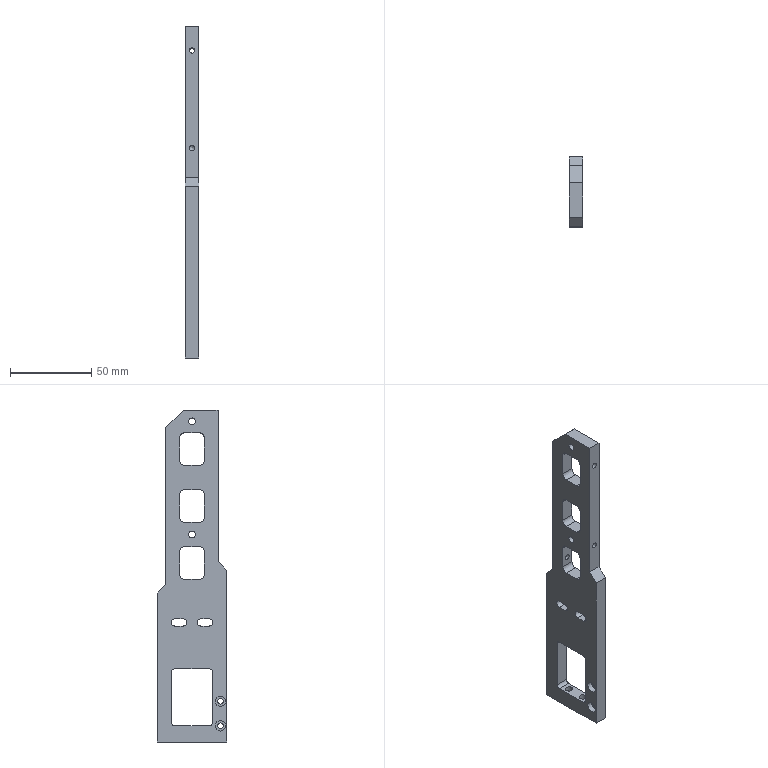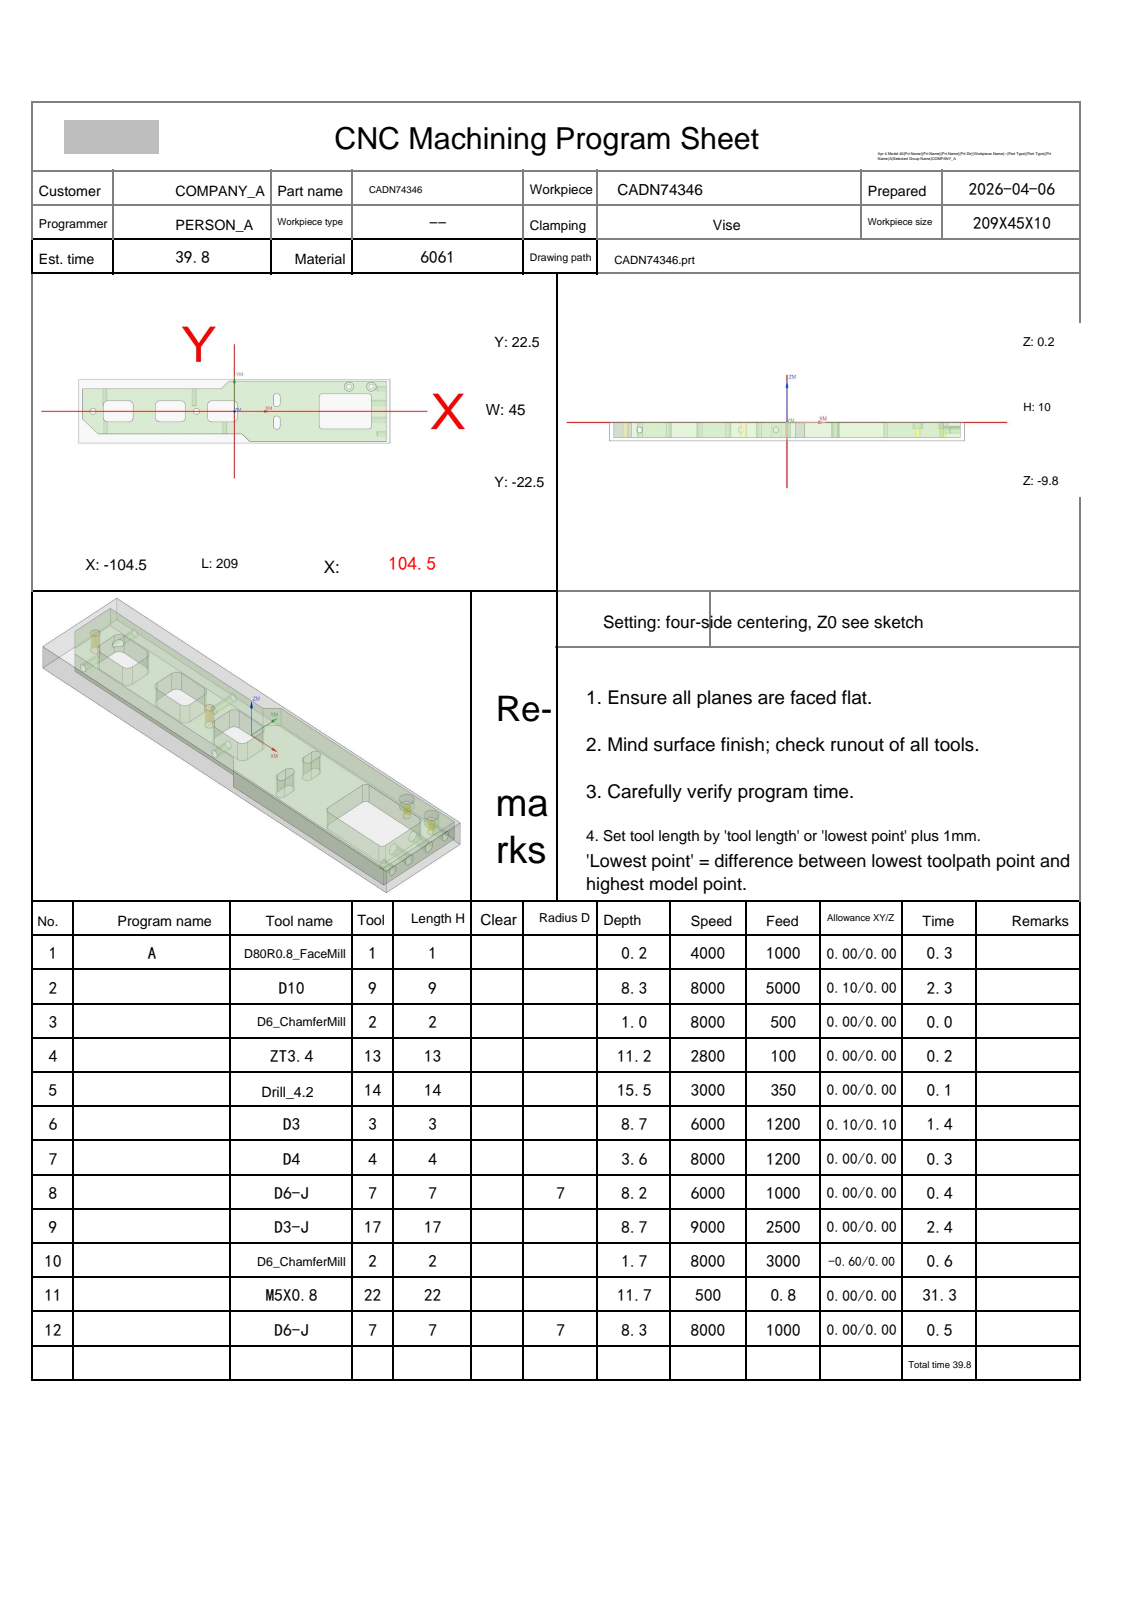NC program | NX | posted by the shop | part box 8 x 43 x 204 mm
Lines 1 to 1524 of 14335, first 1374 of 1522 lines:
%
O0001
(Machine time: 70.91 MIN)
(===Total Tool:10===)
(T1=D80R0.8 FaceMill D=80.  R=0.8  D-  H01 Z=-0.   )
(T9=D10     D=10.  R=0.   D-  H09 Z=-8.1  )
(T2=D6_ChamferMill   D=6.   R=0.   D-  H02 Z=-1.5  )
(T13=ZT3.4  D=3.4  DR_a=118 D-  H13 Z=-11.02)
(T14=Drill 4.2  D=4.2  DR_a=118 D-  H14 Z=-15.26)
(T3=D3      D=3.   R=0.   D-  H03 Z=-8.5  )
(T4=D4      D=4.   R=0.   D4  H04 Z=-3.4  )
(T7=D6-J    D=6.   R=0.   D7  H07 Z=-8.1  )
(T17=D3-J   D=3.   R=0.   D17 H17 Z=-8.5  )
(T22=M5X0.8 D=4.2  DR_a=180 D-  H22 Z=-11.5 )
G80 G90 G17 G49 G40
G91 G28 Z0
M01
N1 T01 M06
(D80R0.8 FaceMill  D=80. R=0.8 H=01 ce=0.00 di=0.00)
G00 G90 G54 X147. Y0.0 M03 S4000
G43 H01 Z20.
M08
Z2.
G01 Z0.0 F1000.
X142.
X-142.
X-147.
Z2.
G00 Z20.
G91 G28 Z0.0
M05
M09
G91 G28 Z0.0
M01
N2 T09 M06
(D10  D=10. R=0. H=09 ce=0.10 di=0.00)
G00 G90 G54 X49.25 Y26.6 M03 S8000
G43 H09 Z20.
M08
Z.5
G01 X102. Z.42 F5000.
G02 X107.1 Y21.5 Z.407 I0.0 J-5.1
G01 Y-21.5 Z.342
G02 X102. Y-26.6 Z.33 I-5.1 J0.0
G01 X10.5 Z.19
G02 X6.894 Y-25.106 Z.184 I0.0 J5.1
G01 X2.888 Y-21.1 Z.175
X-91.5 Z.032
G02 X-95.106 Y-19.606 Z.026 I0.0 J5.1
G01 X-105.606 Y-9.106 Z.003
G02 X-107.1 Y-5.5 Z-.003 I3.606 J3.606
G01 Y16. Z-.036
G02 X-102. Y21.1 Z-.048 I5.1 J0.0
G01 X-11.112 Z-.187
X-7.106 Y25.106 Z-.195
G02 X-3.5 Y26.6 Z-.201 I3.606 J-3.606
G01 X102. Z-.362
G02 X107.1 Y21.5 Z-.374 I0.0 J-5.1
G01 Y-21.5 Z-.44
G02 X102. Y-26.6 Z-.452 I-5.1 J0.0
G01 X10.5 Z-.592
G02 X6.894 Y-25.106 Z-.598 I0.0 J5.1
G01 X2.888 Y-21.1 Z-.606
X-91.5 Z-.75
G02 X-95.106 Y-19.606 Z-.756 I0.0 J5.1
G01 X-105.606 Y-9.106 Z-.779
G02 X-107.1 Y-5.5 Z-.785 I3.606 J3.606
G01 Y16. Z-.818
G02 X-102. Y21.1 Z-.83 I5.1 J0.0
G01 X-11.112 Z-.969
X-7.106 Y25.106 Z-.977
G02 X-3.5 Y26.6 Z-.983 I3.606 J-3.606
G01 X102. Z-1.144
G02 X107.1 Y21.5 Z-1.156 I0.0 J-5.1
G01 Y-21.5 Z-1.222
G02 X102. Y-26.6 Z-1.234 I-5.1 J0.0
G01 X10.5 Z-1.373
G02 X6.894 Y-25.106 Z-1.38 I0.0 J5.1
G01 X2.888 Y-21.1 Z-1.388
X-91.5 Z-1.532
G02 X-95.106 Y-19.606 Z-1.538 I0.0 J5.1
G01 X-105.606 Y-9.106 Z-1.561
G02 X-107.1 Y-5.5 Z-1.567 I3.606 J3.606
G01 Y16. Z-1.6
G02 X-102. Y21.1 Z-1.612 I5.1 J0.0
G01 X-11.112 Z-1.75
X-7.106 Y25.106 Z-1.759
G02 X-3.5 Y26.6 Z-1.765 I3.606 J-3.606
G01 X102. Z-1.926
G02 X107.1 Y21.5 Z-1.938 I0.0 J-5.1
G01 Y-21.5 Z-2.004
G02 X102. Y-26.6 Z-2.016 I-5.1 J0.0
G01 X10.5 Z-2.155
G02 X6.894 Y-25.106 Z-2.161 I0.0 J5.1
G01 X2.888 Y-21.1 Z-2.17
X-91.5 Z-2.314
G02 X-95.106 Y-19.606 Z-2.32 I0.0 J5.1
G01 X-105.606 Y-9.106 Z-2.343
G02 X-107.1 Y-5.5 Z-2.349 I3.606 J3.606
G01 Y16. Z-2.381
G02 X-102. Y21.1 Z-2.394 I5.1 J0.0
G01 X-11.112 Z-2.532
X-7.106 Y25.106 Z-2.541
G02 X-3.5 Y26.6 Z-2.547 I3.606 J-3.606
G01 X102. Z-2.708
G02 X107.1 Y21.5 Z-2.72 I0.0 J-5.1
G01 Y-21.5 Z-2.785
G02 X102. Y-26.6 Z-2.798 I-5.1 J0.0
G01 X10.5 Z-2.937
G02 X6.894 Y-25.106 Z-2.943 I0.0 J5.1
G01 X2.888 Y-21.1 Z-2.952
X-91.5 Z-3.096
G02 X-95.106 Y-19.606 Z-3.102 I0.0 J5.1
G01 X-105.606 Y-9.106 Z-3.124
G02 X-107.1 Y-5.5 Z-3.13 I3.606 J3.606
G01 Y16. Z-3.163
G02 X-102. Y21.1 Z-3.175 I5.1 J0.0
G01 X-11.112 Z-3.314
X-7.106 Y25.106 Z-3.323
G02 X-3.5 Y26.6 Z-3.329 I3.606 J-3.606
G01 X102. Z-3.489
G02 X107.1 Y21.5 Z-3.502 I0.0 J-5.1
G01 Y-21.5 Z-3.567
G02 X102. Y-26.6 Z-3.579 I-5.1 J0.0
G01 X10.5 Z-3.719
G02 X6.894 Y-25.106 Z-3.725 I0.0 J5.1
G01 X2.888 Y-21.1 Z-3.734
X-91.5 Z-3.877
G02 X-95.106 Y-19.606 Z-3.884 I0.0 J5.1
G01 X-105.606 Y-9.106 Z-3.906
G02 X-107.1 Y-5.5 Z-3.912 I3.606 J3.606
G01 Y16. Z-3.945
G02 X-102. Y21.1 Z-3.957 I5.1 J0.0
G01 X-11.112 Z-4.096
X-7.106 Y25.106 Z-4.104
G02 X-3.5 Y26.6 Z-4.111 I3.606 J-3.606
G01 X102. Z-4.271
G02 X107.1 Y21.5 Z-4.284 I0.0 J-5.1
G01 Y-21.5 Z-4.349
G02 X102. Y-26.6 Z-4.361 I-5.1 J0.0
G01 X10.5 Z-4.501
G02 X6.894 Y-25.106 Z-4.507 I0.0 J5.1
G01 X2.888 Y-21.1 Z-4.515
X-91.5 Z-4.659
G02 X-95.106 Y-19.606 Z-4.665 I0.0 J5.1
G01 X-105.606 Y-9.106 Z-4.688
G02 X-107.1 Y-5.5 Z-4.694 I3.606 J3.606
G01 Y16. Z-4.727
G02 X-102. Y21.1 Z-4.739 I5.1 J0.0
G01 X-11.112 Z-4.878
X-7.106 Y25.106 Z-4.886
G02 X-3.5 Y26.6 Z-4.892 I3.606 J-3.606
G01 X102. Z-5.053
G02 X107.1 Y21.5 Z-5.065 I0.0 J-5.1
G01 Y-21.5 Z-5.131
G02 X102. Y-26.6 Z-5.143 I-5.1 J0.0
G01 X10.5 Z-5.283
G02 X6.894 Y-25.106 Z-5.289 I0.0 J5.1
G01 X2.888 Y-21.1 Z-5.297
X-91.5 Z-5.441
G02 X-95.106 Y-19.606 Z-5.447 I0.0 J5.1
G01 X-105.606 Y-9.106 Z-5.47
G02 X-107.1 Y-5.5 Z-5.476 I3.606 J3.606
G01 Y16. Z-5.509
G02 X-102. Y21.1 Z-5.521 I5.1 J0.0
G01 X-11.112 Z-5.659
X-7.106 Y25.106 Z-5.668
G02 X-3.5 Y26.6 Z-5.674 I3.606 J-3.606
G01 X102. Z-5.835
G02 X107.1 Y21.5 Z-5.847 I0.0 J-5.1
G01 Y-21.5 Z-5.913
G02 X102. Y-26.6 Z-5.925 I-5.1 J0.0
G01 X10.5 Z-6.064
G02 X6.894 Y-25.106 Z-6.07 I0.0 J5.1
G01 X2.888 Y-21.1 Z-6.079
X-91.5 Z-6.223
G02 X-95.106 Y-19.606 Z-6.229 I0.0 J5.1
G01 X-105.606 Y-9.106 Z-6.252
G02 X-107.1 Y-5.5 Z-6.258 I3.606 J3.606
G01 Y16. Z-6.291
G02 X-102. Y21.1 Z-6.303 I5.1 J0.0
G01 X-11.112 Z-6.441
X-7.106 Y25.106 Z-6.45
G02 X-3.5 Y26.6 Z-6.456 I3.606 J-3.606
G01 X102. Z-6.617
G02 X107.1 Y21.5 Z-6.629 I0.0 J-5.1
G01 Y-21.5 Z-6.694
G02 X102. Y-26.6 Z-6.707 I-5.1 J0.0
G01 X10.5 Z-6.846
G02 X6.894 Y-25.106 Z-6.852 I0.0 J5.1
G01 X2.888 Y-21.1 Z-6.861
X-91.5 Z-7.005
G02 X-95.106 Y-19.606 Z-7.011 I0.0 J5.1
G01 X-105.606 Y-9.106 Z-7.033
G02 X-107.1 Y-5.5 Z-7.04 I3.606 J3.606
G01 Y16. Z-7.072
G02 X-102. Y21.1 Z-7.085 I5.1 J0.0
G01 X-11.112 Z-7.223
X-7.106 Y25.106 Z-7.232
G02 X-3.5 Y26.6 Z-7.238 I3.606 J-3.606
G01 X102. Z-7.399
G02 X107.1 Y21.5 Z-7.411 I0.0 J-5.1
G01 Y-21.5 Z-7.476
G02 X102. Y-26.6 Z-7.489 I-5.1 J0.0
G01 X10.5 Z-7.628
G02 X6.894 Y-25.106 Z-7.634 I0.0 J5.1
G01 X2.888 Y-21.1 Z-7.643
X-91.5 Z-7.787
G02 X-95.106 Y-19.606 Z-7.793 I0.0 J5.1
G01 X-105.606 Y-9.106 Z-7.815
G02 X-107.1 Y-5.5 Z-7.821 I3.606 J3.606
G01 Y16. Z-7.854
G02 X-102. Y21.1 Z-7.866 I5.1 J0.0
G01 X-11.112 Z-8.005
X-7.106 Y25.106 Z-8.014
G02 X-3.5 Y26.6 Z-8.02 I3.606 J-3.606
G01 X49.25 Z-8.1
X102.
G02 X107.1 Y21.5 I0.0 J-5.1
G01 Y-21.5
G02 X102. Y-26.6 I-5.1 J0.0
G01 X10.5
G02 X6.894 Y-25.106 I0.0 J5.1
G01 X2.888 Y-21.1
X-91.5
G02 X-95.106 Y-19.606 I0.0 J5.1
G01 X-105.606 Y-9.106
G02 X-107.1 Y-5.5 I3.606 J3.606
G01 Y16.
G02 X-102. Y21.1 I5.1 J0.0
G01 X-11.112
X-7.106 Y25.106
G02 X-3.5 Y26.6 I3.606 J-3.606
G01 X49.25
X49.75
Z-7.1
G00 Z20.
G00 G90 X74.5 Y-7.4 M03 S6000
Z20.
Z.5
G01 X86.9 Z.424 F4000.
Y7.4 Z.332
X62.1 Z.179
Y-7.4 Z.088
X86.9 Z-.065
Y7.4 Z-.156
X62.1 Z-.309
Y-7.4 Z-.4
X86.9 Z-.553
Y7.4 Z-.644
X62.1 Z-.797
Y-7.4 Z-.888
X86.9 Z-1.041
Y7.4 Z-1.132
X62.1 Z-1.285
Y-7.4 Z-1.377
X86.9 Z-1.529
Y7.4 Z-1.621
X62.1 Z-1.774
Y-7.4 Z-1.865
X86.9 Z-2.018
Y7.4 Z-2.109
X62.1 Z-2.262
Y-7.4 Z-2.353
X86.9 Z-2.506
Y7.4 Z-2.597
X62.1 Z-2.75
Y-7.4 Z-2.841
X86.9 Z-2.994
Y7.4 Z-3.085
X62.1 Z-3.238
Y-7.4 Z-3.329
X86.9 Z-3.482
Y7.4 Z-3.574
X62.1 Z-3.726
Y-7.4 Z-3.818
X86.9 Z-3.971
Y7.4 Z-4.062
X62.1 Z-4.215
Y-7.4 Z-4.306
X86.9 Z-4.459
Y7.4 Z-4.55
X62.1 Z-4.703
Y-7.4 Z-4.794
X86.9 Z-4.947
Y7.4 Z-5.038
X62.1 Z-5.191
Y-7.4 Z-5.282
X86.9 Z-5.435
Y7.4 Z-5.527
X62.1 Z-5.679
Y-7.4 Z-5.771
X86.9 Z-5.924
Y7.4 Z-6.015
X62.1 Z-6.168
Y-7.4 Z-6.259
X86.9 Z-6.412
Y7.4 Z-6.503
X62.1 Z-6.656
Y-7.4 Z-6.747
X86.9 Z-6.9
Y7.4 Z-6.991
X62.1 Z-7.144
Y-7.4 Z-7.235
X86.9 Z-7.388
Y7.4 Z-7.479
X62.1 Z-7.632
Y-7.4 Z-7.724
X74.5 Z-7.8
X86.9
Y7.4
X62.1
Y-7.4
X74.5
X75.
Z-6.8
G00 Z20.
G00 G90 X-8. Y-2.4 M03 S6000
Z20.
Z.5
G01 X-3.1 Z.416 F2500.
Y2.4 Z.334
X-12.9 Z.166
Y-2.4 Z.084
X-3.1 Z-.084
Y2.4 Z-.166
X-12.9 Z-.334
Y-2.4 Z-.416
X-3.1 Z-.584
Y2.4 Z-.666
X-12.9 Z-.834
Y-2.4 Z-.916
X-3.1 Z-1.084
Y2.4 Z-1.166
X-12.9 Z-1.334
Y-2.4 Z-1.416
X-3.1 Z-1.584
Y2.4 Z-1.666
X-12.9 Z-1.834
Y-2.4 Z-1.916
X-3.1 Z-2.084
Y2.4 Z-2.166
X-12.9 Z-2.334
Y-2.4 Z-2.416
X-3.1 Z-2.584
Y2.4 Z-2.666
X-12.9 Z-2.834
Y-2.4 Z-2.916
X-3.1 Z-3.084
Y2.4 Z-3.166
X-12.9 Z-3.334
Y-2.4 Z-3.416
X-3.1 Z-3.584
Y2.4 Z-3.666
X-12.9 Z-3.834
Y-2.4 Z-3.916
X-3.1 Z-4.084
Y2.4 Z-4.166
X-12.9 Z-4.334
Y-2.4 Z-4.416
X-3.1 Z-4.584
Y2.4 Z-4.666
X-12.9 Z-4.834
Y-2.4 Z-4.916
X-3.1 Z-5.084
Y2.4 Z-5.166
X-12.9 Z-5.334
Y-2.4 Z-5.416
X-3.1 Z-5.584
Y2.4 Z-5.666
X-12.9 Z-5.834
Y-2.4 Z-5.916
X-3.1 Z-6.084
Y2.4 Z-6.166
X-12.9 Z-6.334
Y-2.4 Z-6.416
X-3.1 Z-6.584
Y2.4 Z-6.666
X-12.9 Z-6.834
Y-2.4 Z-6.916
X-3.1 Z-7.084
Y2.4 Z-7.166
X-12.9 Z-7.334
Y-2.4 Z-7.416
X-3.1 Z-7.584
Y2.4 Z-7.666
X-12.9 Z-7.834
Y-2.4 Z-7.916
X-8. Z-8.
X-3.1
Y2.4
X-12.9
Y-2.4
X-8.
X-7.5
Z-7.
G00 Z20.
X-43.
Z.5
G01 X-38.1 Z.416
Y2.4 Z.334
X-47.9 Z.166
Y-2.4 Z.084
X-38.1 Z-.084
Y2.4 Z-.166
X-47.9 Z-.334
Y-2.4 Z-.416
X-38.1 Z-.584
Y2.4 Z-.666
X-47.9 Z-.834
Y-2.4 Z-.916
X-38.1 Z-1.084
Y2.4 Z-1.166
X-47.9 Z-1.334
Y-2.4 Z-1.416
X-38.1 Z-1.584
Y2.4 Z-1.666
X-47.9 Z-1.834
Y-2.4 Z-1.916
X-38.1 Z-2.084
Y2.4 Z-2.166
X-47.9 Z-2.334
Y-2.4 Z-2.416
X-38.1 Z-2.584
Y2.4 Z-2.666
X-47.9 Z-2.834
Y-2.4 Z-2.916
X-38.1 Z-3.084
Y2.4 Z-3.166
X-47.9 Z-3.334
Y-2.4 Z-3.416
X-38.1 Z-3.584
Y2.4 Z-3.666
X-47.9 Z-3.834
Y-2.4 Z-3.916
X-38.1 Z-4.084
Y2.4 Z-4.166
X-47.9 Z-4.334
Y-2.4 Z-4.416
X-38.1 Z-4.584
Y2.4 Z-4.666
X-47.9 Z-4.834
Y-2.4 Z-4.916
X-38.1 Z-5.084
Y2.4 Z-5.166
X-47.9 Z-5.334
Y-2.4 Z-5.416
X-38.1 Z-5.584
Y2.4 Z-5.666
X-47.9 Z-5.834
Y-2.4 Z-5.916
X-38.1 Z-6.084
Y2.4 Z-6.166
X-47.9 Z-6.334
Y-2.4 Z-6.416
X-38.1 Z-6.584
Y2.4 Z-6.666
X-47.9 Z-6.834
Y-2.4 Z-6.916
X-38.1 Z-7.084
Y2.4 Z-7.166
X-47.9 Z-7.334
Y-2.4 Z-7.416
X-38.1 Z-7.584
Y2.4 Z-7.666
X-47.9 Z-7.834
Y-2.4 Z-7.916
X-43. Z-8.
X-38.1
Y2.4
X-47.9
Y-2.4
X-43.
X-42.5
Z-7.
G00 Z20.
X-78.
Z.5
G01 X-73.1 Z.416
Y2.4 Z.334
X-82.9 Z.166
Y-2.4 Z.084
X-73.1 Z-.084
Y2.4 Z-.166
X-82.9 Z-.334
Y-2.4 Z-.416
X-73.1 Z-.584
Y2.4 Z-.666
X-82.9 Z-.834
Y-2.4 Z-.916
X-73.1 Z-1.084
Y2.4 Z-1.166
X-82.9 Z-1.334
Y-2.4 Z-1.416
X-73.1 Z-1.584
Y2.4 Z-1.666
X-82.9 Z-1.834
Y-2.4 Z-1.916
X-73.1 Z-2.084
Y2.4 Z-2.166
X-82.9 Z-2.334
Y-2.4 Z-2.416
X-73.1 Z-2.584
Y2.4 Z-2.666
X-82.9 Z-2.834
Y-2.4 Z-2.916
X-73.1 Z-3.084
Y2.4 Z-3.166
X-82.9 Z-3.334
Y-2.4 Z-3.416
X-73.1 Z-3.584
Y2.4 Z-3.666
X-82.9 Z-3.834
Y-2.4 Z-3.916
X-73.1 Z-4.084
Y2.4 Z-4.166
X-82.9 Z-4.334
Y-2.4 Z-4.416
X-73.1 Z-4.584
Y2.4 Z-4.666
X-82.9 Z-4.834
Y-2.4 Z-4.916
X-73.1 Z-5.084
Y2.4 Z-5.166
X-82.9 Z-5.334
Y-2.4 Z-5.416
X-73.1 Z-5.584
Y2.4 Z-5.666
X-82.9 Z-5.834
Y-2.4 Z-5.916
X-73.1 Z-6.084
Y2.4 Z-6.166
X-82.9 Z-6.334
Y-2.4 Z-6.416
X-73.1 Z-6.584
Y2.4 Z-6.666
X-82.9 Z-6.834
Y-2.4 Z-6.916
X-73.1 Z-7.084
Y2.4 Z-7.166
X-82.9 Z-7.334
Y-2.4 Z-7.416
X-73.1 Z-7.584
Y2.4 Z-7.666
X-82.9 Z-7.834
Y-2.4 Z-7.916
X-78. Z-8.
X-73.1
Y2.4
X-82.9
Y-2.4
X-78.
X-77.5
Z-7.
G00 Z20.
G91 G28 Z0.0
M05
M09
G91 G28 Z0.0
M01
N3 T02 M06
(D6_ChamferMill  D=6. R=0. H=02 ce=0.00 di=0.10)
G00 G90 G54 X-95. Y0.0 M03 S8000
G43 H02 Z20.
M08
G98 G81 X-95. Y0.0 Z-.8 R1. F500.
X-25.5
X77. Y17.5
X92.
G80
G00 Z20.
G91 G28 Z0.0
M05
M09
G91 G28 Z0.0
M01
N4 T13 M06
(ZT3.4 D=3.4 DR_a=118 H=13)
G00 G90 G54 X92. Y17.5 M03 S2800
G43 H13 Z20.
M08
G98 G83 X92. Y17.5 Z-11.021 R1. F100. Q2.
X77.
G80
G00 Z20.
G91 G28 Z0.0
M05
M09
G91 G28 Z0.0
M01
N5 T14 M06
(Drill 4.2 D=4.2 DR_a=118 H=14)
G00 G90 G54 X-95. Y0.0 M03 S3000
G43 H14 Z20.
M08
G98 G83 X-95. Y0.0 Z-15.262 R1. F350. Q3.
X-25.5
G80
G00 Z20.
G91 G28 Z0.0
M05
M09
G91 G28 Z0.0
M01
N6 T03 M06
(D3  D=3. R=0. H=03 ce=0.10 di=0.10)
G00 G90 G54 X29.15 Y-8. M03 S6000
G43 H03 Z20.
M08
Z.5
G01 Y-5.5 Z.473 F1200.
G03 X28.5 Y-4.85 Z.463 I-.65 J0.0
X27.85 Y-5.5 Z.452 I0.0 J-.65
G01 Y-10.5 Z.398
G03 X28.5 Y-11.15 Z.388 I.65 J0.0
X29.15 Y-10.5 Z.377 I0.0 J.65
G01 Y-5.5 Z.323
G03 X28.5 Y-4.85 Z.313 I-.65 J0.0
X27.85 Y-5.5 Z.302 I0.0 J-.65
G01 Y-10.5 Z.248
G03 X28.5 Y-11.15 Z.238 I.65 J0.0
X29.15 Y-10.5 Z.227 I0.0 J.65
G01 Y-5.5 Z.173
G03 X28.5 Y-4.85 Z.163 I-.65 J0.0
X27.85 Y-5.5 Z.152 I0.0 J-.65
G01 Y-10.5 Z.098
G03 X28.5 Y-11.15 Z.088 I.65 J0.0
X29.15 Y-10.5 Z.077 I0.0 J.65
G01 Y-5.5 Z.023
G03 X28.5 Y-4.85 Z.013 I-.65 J0.0
X27.85 Y-5.5 Z.002 I0.0 J-.65
G01 Y-10.5 Z-.052
G03 X28.5 Y-11.15 Z-.063 I.65 J0.0
X29.15 Y-10.5 Z-.073 I0.0 J.65
G01 Y-5.5 Z-.127
G03 X28.5 Y-4.85 Z-.138 I-.65 J0.0
X27.85 Y-5.5 Z-.148 I0.0 J-.65
G01 Y-10.5 Z-.202
G03 X28.5 Y-11.15 Z-.213 I.65 J0.0
X29.15 Y-10.5 Z-.223 I0.0 J.65
G01 Y-5.5 Z-.277
G03 X28.5 Y-4.85 Z-.288 I-.65 J0.0
X27.85 Y-5.5 Z-.298 I0.0 J-.65
G01 Y-10.5 Z-.352
G03 X28.5 Y-11.15 Z-.363 I.65 J0.0
X29.15 Y-10.5 Z-.373 I0.0 J.65
G01 Y-5.5 Z-.427
G03 X28.5 Y-4.85 Z-.438 I-.65 J0.0
X27.85 Y-5.5 Z-.448 I0.0 J-.65
G01 Y-10.5 Z-.502
G03 X28.5 Y-11.15 Z-.513 I.65 J0.0
X29.15 Y-10.5 Z-.523 I0.0 J.65
G01 Y-5.5 Z-.577
G03 X28.5 Y-4.85 Z-.588 I-.65 J0.0
X27.85 Y-5.5 Z-.598 I0.0 J-.65
G01 Y-10.5 Z-.652
G03 X28.5 Y-11.15 Z-.663 I.65 J0.0
X29.15 Y-10.5 Z-.673 I0.0 J.65
G01 Y-5.5 Z-.727
G03 X28.5 Y-4.85 Z-.738 I-.65 J0.0
X27.85 Y-5.5 Z-.748 I0.0 J-.65
G01 Y-10.5 Z-.802
G03 X28.5 Y-11.15 Z-.813 I.65 J0.0
X29.15 Y-10.5 Z-.823 I0.0 J.65
G01 Y-5.5 Z-.877
G03 X28.5 Y-4.85 Z-.888 I-.65 J0.0
X27.85 Y-5.5 Z-.898 I0.0 J-.65
G01 Y-10.5 Z-.952
G03 X28.5 Y-11.15 Z-.963 I.65 J0.0
X29.15 Y-10.5 Z-.973 I0.0 J.65
G01 Y-5.5 Z-1.027
G03 X28.5 Y-4.85 Z-1.038 I-.65 J0.0
X27.85 Y-5.5 Z-1.048 I0.0 J-.65
G01 Y-10.5 Z-1.102
G03 X28.5 Y-11.15 Z-1.113 I.65 J0.0
X29.15 Y-10.5 Z-1.123 I0.0 J.65
G01 Y-5.5 Z-1.177
G03 X28.5 Y-4.85 Z-1.188 I-.65 J0.0
X27.85 Y-5.5 Z-1.198 I0.0 J-.65
G01 Y-10.5 Z-1.252
G03 X28.5 Y-11.15 Z-1.263 I.65 J0.0
X29.15 Y-10.5 Z-1.273 I0.0 J.65
G01 Y-5.5 Z-1.327
G03 X28.5 Y-4.85 Z-1.338 I-.65 J0.0
X27.85 Y-5.5 Z-1.348 I0.0 J-.65
G01 Y-10.5 Z-1.402
G03 X28.5 Y-11.15 Z-1.413 I.65 J0.0
X29.15 Y-10.5 Z-1.423 I0.0 J.65
G01 Y-5.5 Z-1.477
G03 X28.5 Y-4.85 Z-1.488 I-.65 J0.0
X27.85 Y-5.5 Z-1.498 I0.0 J-.65
G01 Y-10.5 Z-1.552
G03 X28.5 Y-11.15 Z-1.563 I.65 J0.0
X29.15 Y-10.5 Z-1.573 I0.0 J.65
G01 Y-5.5 Z-1.627
G03 X28.5 Y-4.85 Z-1.638 I-.65 J0.0
X27.85 Y-5.5 Z-1.648 I0.0 J-.65
G01 Y-10.5 Z-1.702
G03 X28.5 Y-11.15 Z-1.713 I.65 J0.0
X29.15 Y-10.5 Z-1.723 I0.0 J.65
G01 Y-5.5 Z-1.777
G03 X28.5 Y-4.85 Z-1.788 I-.65 J0.0
X27.85 Y-5.5 Z-1.798 I0.0 J-.65
G01 Y-10.5 Z-1.852
G03 X28.5 Y-11.15 Z-1.863 I.65 J0.0
X29.15 Y-10.5 Z-1.873 I0.0 J.65
G01 Y-5.5 Z-1.927
G03 X28.5 Y-4.85 Z-1.938 I-.65 J0.0
X27.85 Y-5.5 Z-1.948 I0.0 J-.65
G01 Y-10.5 Z-2.002
G03 X28.5 Y-11.15 Z-2.013 I.65 J0.0
X29.15 Y-10.5 Z-2.023 I0.0 J.65
G01 Y-5.5 Z-2.077
G03 X28.5 Y-4.85 Z-2.088 I-.65 J0.0
X27.85 Y-5.5 Z-2.098 I0.0 J-.65
G01 Y-10.5 Z-2.152
G03 X28.5 Y-11.15 Z-2.163 I.65 J0.0
X29.15 Y-10.5 Z-2.173 I0.0 J.65
G01 Y-5.5 Z-2.227
G03 X28.5 Y-4.85 Z-2.238 I-.65 J0.0
X27.85 Y-5.5 Z-2.248 I0.0 J-.65
G01 Y-10.5 Z-2.302
G03 X28.5 Y-11.15 Z-2.313 I.65 J0.0
X29.15 Y-10.5 Z-2.323 I0.0 J.65
G01 Y-5.5 Z-2.377
G03 X28.5 Y-4.85 Z-2.388 I-.65 J0.0
X27.85 Y-5.5 Z-2.398 I0.0 J-.65
G01 Y-10.5 Z-2.452
G03 X28.5 Y-11.15 Z-2.463 I.65 J0.0
X29.15 Y-10.5 Z-2.473 I0.0 J.65
G01 Y-5.5 Z-2.527
G03 X28.5 Y-4.85 Z-2.538 I-.65 J0.0
X27.85 Y-5.5 Z-2.548 I0.0 J-.65
G01 Y-10.5 Z-2.602
G03 X28.5 Y-11.15 Z-2.613 I.65 J0.0
X29.15 Y-10.5 Z-2.623 I0.0 J.65
G01 Y-5.5 Z-2.677
G03 X28.5 Y-4.85 Z-2.688 I-.65 J0.0
X27.85 Y-5.5 Z-2.698 I0.0 J-.65
G01 Y-10.5 Z-2.752
G03 X28.5 Y-11.15 Z-2.763 I.65 J0.0
X29.15 Y-10.5 Z-2.773 I0.0 J.65
G01 Y-5.5 Z-2.827
G03 X28.5 Y-4.85 Z-2.838 I-.65 J0.0
X27.85 Y-5.5 Z-2.848 I0.0 J-.65
G01 Y-10.5 Z-2.902
G03 X28.5 Y-11.15 Z-2.913 I.65 J0.0
X29.15 Y-10.5 Z-2.923 I0.0 J.65
G01 Y-5.5 Z-2.977
G03 X28.5 Y-4.85 Z-2.988 I-.65 J0.0
X27.85 Y-5.5 Z-2.998 I0.0 J-.65
G01 Y-10.5 Z-3.052
G03 X28.5 Y-11.15 Z-3.063 I.65 J0.0
X29.15 Y-10.5 Z-3.073 I0.0 J.65
G01 Y-5.5 Z-3.127
G03 X28.5 Y-4.85 Z-3.138 I-.65 J0.0
X27.85 Y-5.5 Z-3.148 I0.0 J-.65
G01 Y-10.5 Z-3.202
G03 X28.5 Y-11.15 Z-3.213 I.65 J0.0
X29.15 Y-10.5 Z-3.223 I0.0 J.65
G01 Y-5.5 Z-3.277
G03 X28.5 Y-4.85 Z-3.288 I-.65 J0.0
X27.85 Y-5.5 Z-3.298 I0.0 J-.65
G01 Y-10.5 Z-3.352
G03 X28.5 Y-11.15 Z-3.363 I.65 J0.0
X29.15 Y-10.5 Z-3.373 I0.0 J.65
G01 Y-5.5 Z-3.427
G03 X28.5 Y-4.85 Z-3.438 I-.65 J0.0
X27.85 Y-5.5 Z-3.448 I0.0 J-.65
G01 Y-10.5 Z-3.502
G03 X28.5 Y-11.15 Z-3.513 I.65 J0.0
X29.15 Y-10.5 Z-3.523 I0.0 J.65
G01 Y-5.5 Z-3.577
G03 X28.5 Y-4.85 Z-3.588 I-.65 J0.0
X27.85 Y-5.5 Z-3.598 I0.0 J-.65
G01 Y-10.5 Z-3.652
G03 X28.5 Y-11.15 Z-3.663 I.65 J0.0
X29.15 Y-10.5 Z-3.673 I0.0 J.65
G01 Y-5.5 Z-3.727
G03 X28.5 Y-4.85 Z-3.738 I-.65 J0.0
X27.85 Y-5.5 Z-3.748 I0.0 J-.65
G01 Y-10.5 Z-3.802
G03 X28.5 Y-11.15 Z-3.813 I.65 J0.0
X29.15 Y-10.5 Z-3.823 I0.0 J.65
G01 Y-5.5 Z-3.877
G03 X28.5 Y-4.85 Z-3.888 I-.65 J0.0
X27.85 Y-5.5 Z-3.898 I0.0 J-.65
G01 Y-10.5 Z-3.952
G03 X28.5 Y-11.15 Z-3.963 I.65 J0.0
X29.15 Y-10.5 Z-3.973 I0.0 J.65
G01 Y-5.5 Z-4.027
G03 X28.5 Y-4.85 Z-4.038 I-.65 J0.0
X27.85 Y-5.5 Z-4.048 I0.0 J-.65
G01 Y-10.5 Z-4.102
G03 X28.5 Y-11.15 Z-4.113 I.65 J0.0
X29.15 Y-10.5 Z-4.123 I0.0 J.65
G01 Y-5.5 Z-4.177
G03 X28.5 Y-4.85 Z-4.188 I-.65 J0.0
X27.85 Y-5.5 Z-4.198 I0.0 J-.65
G01 Y-10.5 Z-4.252
G03 X28.5 Y-11.15 Z-4.263 I.65 J0.0
X29.15 Y-10.5 Z-4.273 I0.0 J.65
G01 Y-5.5 Z-4.327
G03 X28.5 Y-4.85 Z-4.338 I-.65 J0.0
X27.85 Y-5.5 Z-4.348 I0.0 J-.65
G01 Y-10.5 Z-4.402
G03 X28.5 Y-11.15 Z-4.413 I.65 J0.0
X29.15 Y-10.5 Z-4.423 I0.0 J.65
G01 Y-5.5 Z-4.477
G03 X28.5 Y-4.85 Z-4.488 I-.65 J0.0
X27.85 Y-5.5 Z-4.498 I0.0 J-.65
G01 Y-10.5 Z-4.552
G03 X28.5 Y-11.15 Z-4.563 I.65 J0.0
X29.15 Y-10.5 Z-4.573 I0.0 J.65
G01 Y-5.5 Z-4.627
G03 X28.5 Y-4.85 Z-4.638 I-.65 J0.0
X27.85 Y-5.5 Z-4.648 I0.0 J-.65
G01 Y-10.5 Z-4.702
G03 X28.5 Y-11.15 Z-4.713 I.65 J0.0
X29.15 Y-10.5 Z-4.723 I0.0 J.65
G01 Y-5.5 Z-4.777
G03 X28.5 Y-4.85 Z-4.788 I-.65 J0.0
X27.85 Y-5.5 Z-4.798 I0.0 J-.65
G01 Y-10.5 Z-4.852
G03 X28.5 Y-11.15 Z-4.863 I.65 J0.0
X29.15 Y-10.5 Z-4.873 I0.0 J.65
G01 Y-5.5 Z-4.927
G03 X28.5 Y-4.85 Z-4.938 I-.65 J0.0
X27.85 Y-5.5 Z-4.948 I0.0 J-.65
G01 Y-10.5 Z-5.002
G03 X28.5 Y-11.15 Z-5.013 I.65 J0.0
X29.15 Y-10.5 Z-5.023 I0.0 J.65
G01 Y-5.5 Z-5.077
G03 X28.5 Y-4.85 Z-5.088 I-.65 J0.0
X27.85 Y-5.5 Z-5.098 I0.0 J-.65
G01 Y-10.5 Z-5.152
G03 X28.5 Y-11.15 Z-5.163 I.65 J0.0
X29.15 Y-10.5 Z-5.173 I0.0 J.65
G01 Y-5.5 Z-5.227
G03 X28.5 Y-4.85 Z-5.238 I-.65 J0.0
X27.85 Y-5.5 Z-5.248 I0.0 J-.65
G01 Y-10.5 Z-5.302
G03 X28.5 Y-11.15 Z-5.313 I.65 J0.0
X29.15 Y-10.5 Z-5.323 I0.0 J.65
G01 Y-5.5 Z-5.377
G03 X28.5 Y-4.85 Z-5.388 I-.65 J0.0
X27.85 Y-5.5 Z-5.398 I0.0 J-.65
G01 Y-10.5 Z-5.452
G03 X28.5 Y-11.15 Z-5.463 I.65 J0.0
X29.15 Y-10.5 Z-5.473 I0.0 J.65
G01 Y-5.5 Z-5.527
G03 X28.5 Y-4.85 Z-5.538 I-.65 J0.0
X27.85 Y-5.5 Z-5.548 I0.0 J-.65
G01 Y-10.5 Z-5.602
G03 X28.5 Y-11.15 Z-5.613 I.65 J0.0
X29.15 Y-10.5 Z-5.623 I0.0 J.65
G01 Y-5.5 Z-5.677
G03 X28.5 Y-4.85 Z-5.688 I-.65 J0.0
X27.85 Y-5.5 Z-5.698 I0.0 J-.65
G01 Y-10.5 Z-5.752
G03 X28.5 Y-11.15 Z-5.763 I.65 J0.0
X29.15 Y-10.5 Z-5.773 I0.0 J.65
G01 Y-5.5 Z-5.827
G03 X28.5 Y-4.85 Z-5.838 I-.65 J0.0
X27.85 Y-5.5 Z-5.848 I0.0 J-.65
G01 Y-10.5 Z-5.902
G03 X28.5 Y-11.15 Z-5.913 I.65 J0.0
X29.15 Y-10.5 Z-5.923 I0.0 J.65
G01 Y-5.5 Z-5.977
G03 X28.5 Y-4.85 Z-5.988 I-.65 J0.0
X27.85 Y-5.5 Z-5.998 I0.0 J-.65
G01 Y-10.5 Z-6.052
G03 X28.5 Y-11.15 Z-6.063 I.65 J0.0
X29.15 Y-10.5 Z-6.073 I0.0 J.65
G01 Y-5.5 Z-6.127
G03 X28.5 Y-4.85 Z-6.138 I-.65 J0.0
X27.85 Y-5.5 Z-6.148 I0.0 J-.65
G01 Y-10.5 Z-6.202
G03 X28.5 Y-11.15 Z-6.213 I.65 J0.0
X29.15 Y-10.5 Z-6.223 I0.0 J.65
G01 Y-5.5 Z-6.277
G03 X28.5 Y-4.85 Z-6.288 I-.65 J0.0
X27.85 Y-5.5 Z-6.298 I0.0 J-.65
G01 Y-10.5 Z-6.352
G03 X28.5 Y-11.15 Z-6.363 I.65 J0.0
X29.15 Y-10.5 Z-6.373 I0.0 J.65
G01 Y-5.5 Z-6.427
G03 X28.5 Y-4.85 Z-6.438 I-.65 J0.0
X27.85 Y-5.5 Z-6.448 I0.0 J-.65
G01 Y-10.5 Z-6.502
G03 X28.5 Y-11.15 Z-6.513 I.65 J0.0
X29.15 Y-10.5 Z-6.523 I0.0 J.65
G01 Y-5.5 Z-6.577
G03 X28.5 Y-4.85 Z-6.588 I-.65 J0.0
X27.85 Y-5.5 Z-6.598 I0.0 J-.65
G01 Y-10.5 Z-6.652
G03 X28.5 Y-11.15 Z-6.663 I.65 J0.0
X29.15 Y-10.5 Z-6.673 I0.0 J.65
G01 Y-5.5 Z-6.727
G03 X28.5 Y-4.85 Z-6.738 I-.65 J0.0
X27.85 Y-5.5 Z-6.748 I0.0 J-.65
G01 Y-10.5 Z-6.802
G03 X28.5 Y-11.15 Z-6.813 I.65 J0.0
X29.15 Y-10.5 Z-6.823 I0.0 J.65
G01 Y-5.5 Z-6.877
G03 X28.5 Y-4.85 Z-6.888 I-.65 J0.0
X27.85 Y-5.5 Z-6.898 I0.0 J-.65
G01 Y-10.5 Z-6.952
G03 X28.5 Y-11.15 Z-6.963 I.65 J0.0
X29.15 Y-10.5 Z-6.973 I0.0 J.65
G01 Y-5.5 Z-7.027
G03 X28.5 Y-4.85 Z-7.038 I-.65 J0.0
X27.85 Y-5.5 Z-7.048 I0.0 J-.65
G01 Y-10.5 Z-7.102
G03 X28.5 Y-11.15 Z-7.113 I.65 J0.0
X29.15 Y-10.5 Z-7.123 I0.0 J.65
G01 Y-5.5 Z-7.177
G03 X28.5 Y-4.85 Z-7.188 I-.65 J0.0
X27.85 Y-5.5 Z-7.198 I0.0 J-.65
G01 Y-10.5 Z-7.252
G03 X28.5 Y-11.15 Z-7.263 I.65 J0.0
X29.15 Y-10.5 Z-7.273 I0.0 J.65
G01 Y-5.5 Z-7.327
G03 X28.5 Y-4.85 Z-7.338 I-.65 J0.0
X27.85 Y-5.5 Z-7.348 I0.0 J-.65
G01 Y-10.5 Z-7.402
G03 X28.5 Y-11.15 Z-7.413 I.65 J0.0
X29.15 Y-10.5 Z-7.423 I0.0 J.65
G01 Y-5.5 Z-7.477
G03 X28.5 Y-4.85 Z-7.488 I-.65 J0.0
X27.85 Y-5.5 Z-7.498 I0.0 J-.65
G01 Y-10.5 Z-7.552
G03 X28.5 Y-11.15 Z-7.563 I.65 J0.0
X29.15 Y-10.5 Z-7.573 I0.0 J.65
G01 Y-5.5 Z-7.627
G03 X28.5 Y-4.85 Z-7.638 I-.65 J0.0
X27.85 Y-5.5 Z-7.648 I0.0 J-.65
G01 Y-10.5 Z-7.702
G03 X28.5 Y-11.15 Z-7.713 I.65 J0.0
X29.15 Y-10.5 Z-7.723 I0.0 J.65
G01 Y-5.5 Z-7.777
G03 X28.5 Y-4.85 Z-7.788 I-.65 J0.0
X27.85 Y-5.5 Z-7.798 I0.0 J-.65
G01 Y-10.5 Z-7.852
G03 X28.5 Y-11.15 Z-7.863 I.65 J0.0
X29.15 Y-10.5 Z-7.873 I0.0 J.65
G01 Y-5.5 Z-7.927
G03 X28.5 Y-4.85 Z-7.938 I-.65 J0.0
X27.85 Y-5.5 Z-7.948 I0.0 J-.65
G01 Y-10.5 Z-8.002
G03 X28.5 Y-11.15 Z-8.013 I.65 J0.0
X29.15 Y-10.5 Z-8.023 I0.0 J.65
G01 Y-5.5 Z-8.077
G03 X28.5 Y-4.85 Z-8.088 I-.65 J0.0
X27.85 Y-5.5 Z-8.098 I0.0 J-.65
G01 Y-10.5 Z-8.152
G03 X28.5 Y-11.15 Z-8.163 I.65 J0.0
X29.15 Y-10.5 Z-8.173 I0.0 J.65
G01 Y-5.5 Z-8.227
G03 X28.5 Y-4.85 Z-8.238 I-.65 J0.0
X27.85 Y-5.5 Z-8.248 I0.0 J-.65
G01 Y-10.5 Z-8.302
G03 X28.5 Y-11.15 Z-8.313 I.65 J0.0
X29.15 Y-10.5 Z-8.323 I0.0 J.65
G01 Y-5.5 Z-8.377
G03 X28.5 Y-4.85 Z-8.388 I-.65 J0.0
X27.85 Y-5.5 Z-8.398 I0.0 J-.65
G01 Y-10.5 Z-8.452
G03 X28.5 Y-11.15 Z-8.463 I.65 J0.0
X29.15 Y-10.5 Z-8.473 I0.0 J.65
G01 Y-8. Z-8.5
Y-5.5
G03 X28.5 Y-4.85 I-.65 J0.0
X27.85 Y-5.5 I0.0 J-.65
G01 Y-10.5
G03 X28.5 Y-11.15 I.65 J0.0
X29.15 Y-10.5 I0.0 J.65
G01 Y-8.
Y-7.5
Z-7.5
G00 Z20.
Y8.
Z.5
G01 Y10.5 Z.473
G03 X28.5 Y11.15 Z.463 I-.65 J0.0
X27.85 Y10.5 Z.452 I0.0 J-.65
G01 Y5.5 Z.398
G03 X28.5 Y4.85 Z.388 I.65 J0.0
X29.15 Y5.5 Z.377 I0.0 J.65
G01 Y10.5 Z.323
G03 X28.5 Y11.15 Z.313 I-.65 J0.0
X27.85 Y10.5 Z.302 I0.0 J-.65
G01 Y5.5 Z.248
G03 X28.5 Y4.85 Z.238 I.65 J0.0
X29.15 Y5.5 Z.227 I0.0 J.65
G01 Y10.5 Z.173
G03 X28.5 Y11.15 Z.163 I-.65 J0.0
X27.85 Y10.5 Z.152 I0.0 J-.65
G01 Y5.5 Z.098
G03 X28.5 Y4.85 Z.088 I.65 J0.0
X29.15 Y5.5 Z.077 I0.0 J.65
G01 Y10.5 Z.023
G03 X28.5 Y11.15 Z.013 I-.65 J0.0
X27.85 Y10.5 Z.002 I0.0 J-.65
G01 Y5.5 Z-.052
G03 X28.5 Y4.85 Z-.063 I.65 J0.0
X29.15 Y5.5 Z-.073 I0.0 J.65
G01 Y10.5 Z-.127
G03 X28.5 Y11.15 Z-.138 I-.65 J0.0
X27.85 Y10.5 Z-.148 I0.0 J-.65
G01 Y5.5 Z-.202
G03 X28.5 Y4.85 Z-.213 I.65 J0.0
X29.15 Y5.5 Z-.223 I0.0 J.65
G01 Y10.5 Z-.277
G03 X28.5 Y11.15 Z-.288 I-.65 J0.0
X27.85 Y10.5 Z-.298 I0.0 J-.65
G01 Y5.5 Z-.352
G03 X28.5 Y4.85 Z-.363 I.65 J0.0
X29.15 Y5.5 Z-.373 I0.0 J.65
G01 Y10.5 Z-.427
G03 X28.5 Y11.15 Z-.438 I-.65 J0.0
X27.85 Y10.5 Z-.448 I0.0 J-.65
G01 Y5.5 Z-.502
G03 X28.5 Y4.85 Z-.513 I.65 J0.0
X29.15 Y5.5 Z-.523 I0.0 J.65
G01 Y10.5 Z-.577
G03 X28.5 Y11.15 Z-.588 I-.65 J0.0
X27.85 Y10.5 Z-.598 I0.0 J-.65
G01 Y5.5 Z-.652
G03 X28.5 Y4.85 Z-.663 I.65 J0.0
X29.15 Y5.5 Z-.673 I0.0 J.65
G01 Y10.5 Z-.727
G03 X28.5 Y11.15 Z-.738 I-.65 J0.0
X27.85 Y10.5 Z-.748 I0.0 J-.65
G01 Y5.5 Z-.802
G03 X28.5 Y4.85 Z-.813 I.65 J0.0
X29.15 Y5.5 Z-.823 I0.0 J.65
G01 Y10.5 Z-.877
G03 X28.5 Y11.15 Z-.888 I-.65 J0.0
X27.85 Y10.5 Z-.898 I0.0 J-.65
G01 Y5.5 Z-.952
G03 X28.5 Y4.85 Z-.963 I.65 J0.0
X29.15 Y5.5 Z-.973 I0.0 J.65
G01 Y10.5 Z-1.027
G03 X28.5 Y11.15 Z-1.038 I-.65 J0.0
X27.85 Y10.5 Z-1.048 I0.0 J-.65
G01 Y5.5 Z-1.102
G03 X28.5 Y4.85 Z-1.113 I.65 J0.0
X29.15 Y5.5 Z-1.123 I0.0 J.65
G01 Y10.5 Z-1.177
G03 X28.5 Y11.15 Z-1.188 I-.65 J0.0
X27.85 Y10.5 Z-1.198 I0.0 J-.65
G01 Y5.5 Z-1.252
G03 X28.5 Y4.85 Z-1.263 I.65 J0.0
X29.15 Y5.5 Z-1.273 I0.0 J.65
G01 Y10.5 Z-1.327
G03 X28.5 Y11.15 Z-1.338 I-.65 J0.0
X27.85 Y10.5 Z-1.348 I0.0 J-.65
G01 Y5.5 Z-1.402
G03 X28.5 Y4.85 Z-1.413 I.65 J0.0
X29.15 Y5.5 Z-1.423 I0.0 J.65
G01 Y10.5 Z-1.477
G03 X28.5 Y11.15 Z-1.488 I-.65 J0.0
X27.85 Y10.5 Z-1.498 I0.0 J-.65
G01 Y5.5 Z-1.552
G03 X28.5 Y4.85 Z-1.563 I.65 J0.0
X29.15 Y5.5 Z-1.573 I0.0 J.65
G01 Y10.5 Z-1.627
G03 X28.5 Y11.15 Z-1.638 I-.65 J0.0
X27.85 Y10.5 Z-1.648 I0.0 J-.65
G01 Y5.5 Z-1.702
G03 X28.5 Y4.85 Z-1.713 I.65 J0.0
X29.15 Y5.5 Z-1.723 I0.0 J.65
G01 Y10.5 Z-1.777
G03 X28.5 Y11.15 Z-1.788 I-.65 J0.0
X27.85 Y10.5 Z-1.798 I0.0 J-.65
G01 Y5.5 Z-1.852
G03 X28.5 Y4.85 Z-1.863 I.65 J0.0
X29.15 Y5.5 Z-1.873 I0.0 J.65
G01 Y10.5 Z-1.927
G03 X28.5 Y11.15 Z-1.938 I-.65 J0.0
X27.85 Y10.5 Z-1.948 I0.0 J-.65
G01 Y5.5 Z-2.002
G03 X28.5 Y4.85 Z-2.013 I.65 J0.0
X29.15 Y5.5 Z-2.023 I0.0 J.65
G01 Y10.5 Z-2.077
G03 X28.5 Y11.15 Z-2.088 I-.65 J0.0
X27.85 Y10.5 Z-2.098 I0.0 J-.65
G01 Y5.5 Z-2.152
G03 X28.5 Y4.85 Z-2.163 I.65 J0.0
X29.15 Y5.5 Z-2.173 I0.0 J.65
G01 Y10.5 Z-2.227
G03 X28.5 Y11.15 Z-2.238 I-.65 J0.0
X27.85 Y10.5 Z-2.248 I0.0 J-.65
G01 Y5.5 Z-2.302
G03 X28.5 Y4.85 Z-2.313 I.65 J0.0
X29.15 Y5.5 Z-2.323 I0.0 J.65
G01 Y10.5 Z-2.377
G03 X28.5 Y11.15 Z-2.388 I-.65 J0.0
X27.85 Y10.5 Z-2.398 I0.0 J-.65
G01 Y5.5 Z-2.452
G03 X28.5 Y4.85 Z-2.463 I.65 J0.0
X29.15 Y5.5 Z-2.473 I0.0 J.65
G01 Y10.5 Z-2.527
G03 X28.5 Y11.15 Z-2.538 I-.65 J0.0
X27.85 Y10.5 Z-2.548 I0.0 J-.65
G01 Y5.5 Z-2.602
G03 X28.5 Y4.85 Z-2.613 I.65 J0.0
X29.15 Y5.5 Z-2.623 I0.0 J.65
G01 Y10.5 Z-2.677
G03 X28.5 Y11.15 Z-2.688 I-.65 J0.0
X27.85 Y10.5 Z-2.698 I0.0 J-.65
G01 Y5.5 Z-2.752
G03 X28.5 Y4.85 Z-2.763 I.65 J0.0
X29.15 Y5.5 Z-2.773 I0.0 J.65
G01 Y10.5 Z-2.827
G03 X28.5 Y11.15 Z-2.838 I-.65 J0.0
X27.85 Y10.5 Z-2.848 I0.0 J-.65
G01 Y5.5 Z-2.902
G03 X28.5 Y4.85 Z-2.913 I.65 J0.0
X29.15 Y5.5 Z-2.923 I0.0 J.65
G01 Y10.5 Z-2.977
G03 X28.5 Y11.15 Z-2.988 I-.65 J0.0
X27.85 Y10.5 Z-2.998 I0.0 J-.65
G01 Y5.5 Z-3.052
G03 X28.5 Y4.85 Z-3.063 I.65 J0.0
X29.15 Y5.5 Z-3.073 I0.0 J.65
G01 Y10.5 Z-3.127
G03 X28.5 Y11.15 Z-3.138 I-.65 J0.0
X27.85 Y10.5 Z-3.148 I0.0 J-.65
G01 Y5.5 Z-3.202
G03 X28.5 Y4.85 Z-3.213 I.65 J0.0
X29.15 Y5.5 Z-3.223 I0.0 J.65
G01 Y10.5 Z-3.277
G03 X28.5 Y11.15 Z-3.288 I-.65 J0.0
X27.85 Y10.5 Z-3.298 I0.0 J-.65
G01 Y5.5 Z-3.352
G03 X28.5 Y4.85 Z-3.363 I.65 J0.0
X29.15 Y5.5 Z-3.373 I0.0 J.65
G01 Y10.5 Z-3.427
G03 X28.5 Y11.15 Z-3.438 I-.65 J0.0
X27.85 Y10.5 Z-3.448 I0.0 J-.65
G01 Y5.5 Z-3.502
G03 X28.5 Y4.85 Z-3.513 I.65 J0.0
X29.15 Y5.5 Z-3.523 I0.0 J.65
G01 Y10.5 Z-3.577
G03 X28.5 Y11.15 Z-3.588 I-.65 J0.0
X27.85 Y10.5 Z-3.598 I0.0 J-.65
G01 Y5.5 Z-3.652
G03 X28.5 Y4.85 Z-3.663 I.65 J0.0
X29.15 Y5.5 Z-3.673 I0.0 J.65
G01 Y10.5 Z-3.727
G03 X28.5 Y11.15 Z-3.738 I-.65 J0.0
X27.85 Y10.5 Z-3.748 I0.0 J-.65
G01 Y5.5 Z-3.802
G03 X28.5 Y4.85 Z-3.813 I.65 J0.0
X29.15 Y5.5 Z-3.823 I0.0 J.65
G01 Y10.5 Z-3.877
G03 X28.5 Y11.15 Z-3.888 I-.65 J0.0
X27.85 Y10.5 Z-3.898 I0.0 J-.65
G01 Y5.5 Z-3.952
G03 X28.5 Y4.85 Z-3.963 I.65 J0.0
X29.15 Y5.5 Z-3.973 I0.0 J.65
G01 Y10.5 Z-4.027
G03 X28.5 Y11.15 Z-4.038 I-.65 J0.0
X27.85 Y10.5 Z-4.048 I0.0 J-.65
G01 Y5.5 Z-4.102
G03 X28.5 Y4.85 Z-4.113 I.65 J0.0
X29.15 Y5.5 Z-4.123 I0.0 J.65
G01 Y10.5 Z-4.177
G03 X28.5 Y11.15 Z-4.188 I-.65 J0.0
X27.85 Y10.5 Z-4.198 I0.0 J-.65
G01 Y5.5 Z-4.252
G03 X28.5 Y4.85 Z-4.263 I.65 J0.0
X29.15 Y5.5 Z-4.273 I0.0 J.65
G01 Y10.5 Z-4.327
G03 X28.5 Y11.15 Z-4.338 I-.65 J0.0
X27.85 Y10.5 Z-4.348 I0.0 J-.65
G01 Y5.5 Z-4.402
G03 X28.5 Y4.85 Z-4.413 I.65 J0.0
X29.15 Y5.5 Z-4.423 I0.0 J.65
G01 Y10.5 Z-4.477
G03 X28.5 Y11.15 Z-4.488 I-.65 J0.0
X27.85 Y10.5 Z-4.498 I0.0 J-.65
G01 Y5.5 Z-4.552
G03 X28.5 Y4.85 Z-4.563 I.65 J0.0
X29.15 Y5.5 Z-4.573 I0.0 J.65
G01 Y10.5 Z-4.627
G03 X28.5 Y11.15 Z-4.638 I-.65 J0.0
X27.85 Y10.5 Z-4.648 I0.0 J-.65
G01 Y5.5 Z-4.702
G03 X28.5 Y4.85 Z-4.713 I.65 J0.0
X29.15 Y5.5 Z-4.723 I0.0 J.65
G01 Y10.5 Z-4.777
G03 X28.5 Y11.15 Z-4.788 I-.65 J0.0
X27.85 Y10.5 Z-4.798 I0.0 J-.65
G01 Y5.5 Z-4.852
G03 X28.5 Y4.85 Z-4.863 I.65 J0.0
X29.15 Y5.5 Z-4.873 I0.0 J.65
G01 Y10.5 Z-4.927
G03 X28.5 Y11.15 Z-4.938 I-.65 J0.0
X27.85 Y10.5 Z-4.948 I0.0 J-.65
G01 Y5.5 Z-5.002
G03 X28.5 Y4.85 Z-5.013 I.65 J0.0
X29.15 Y5.5 Z-5.023 I0.0 J.65
G01 Y10.5 Z-5.077
G03 X28.5 Y11.15 Z-5.088 I-.65 J0.0
X27.85 Y10.5 Z-5.098 I0.0 J-.65
G01 Y5.5 Z-5.152
G03 X28.5 Y4.85 Z-5.163 I.65 J0.0
X29.15 Y5.5 Z-5.173 I0.0 J.65
G01 Y10.5 Z-5.227
G03 X28.5 Y11.15 Z-5.238 I-.65 J0.0
X27.85 Y10.5 Z-5.248 I0.0 J-.65
G01 Y5.5 Z-5.302
G03 X28.5 Y4.85 Z-5.313 I.65 J0.0
X29.15 Y5.5 Z-5.323 I0.0 J.65
G01 Y10.5 Z-5.377
G03 X28.5 Y11.15 Z-5.388 I-.65 J0.0
X27.85 Y10.5 Z-5.398 I0.0 J-.65
G01 Y5.5 Z-5.452
G03 X28.5 Y4.85 Z-5.463 I.65 J0.0
X29.15 Y5.5 Z-5.473 I0.0 J.65
G01 Y10.5 Z-5.527
G03 X28.5 Y11.15 Z-5.538 I-.65 J0.0
X27.85 Y10.5 Z-5.548 I0.0 J-.65
G01 Y5.5 Z-5.602
G03 X28.5 Y4.85 Z-5.613 I.65 J0.0
X29.15 Y5.5 Z-5.623 I0.0 J.65
G01 Y10.5 Z-5.677
G03 X28.5 Y11.15 Z-5.688 I-.65 J0.0
X27.85 Y10.5 Z-5.698 I0.0 J-.65
G01 Y5.5 Z-5.752
G03 X28.5 Y4.85 Z-5.763 I.65 J0.0
X29.15 Y5.5 Z-5.773 I0.0 J.65
G01 Y10.5 Z-5.827
G03 X28.5 Y11.15 Z-5.838 I-.65 J0.0
X27.85 Y10.5 Z-5.848 I0.0 J-.65
G01 Y5.5 Z-5.902
G03 X28.5 Y4.85 Z-5.913 I.65 J0.0
X29.15 Y5.5 Z-5.923 I0.0 J.65
G01 Y10.5 Z-5.977
G03 X28.5 Y11.15 Z-5.988 I-.65 J0.0
X27.85 Y10.5 Z-5.998 I0.0 J-.65
G01 Y5.5 Z-6.052
G03 X28.5 Y4.85 Z-6.063 I.65 J0.0
X29.15 Y5.5 Z-6.073 I0.0 J.65
G01 Y10.5 Z-6.127
G03 X28.5 Y11.15 Z-6.138 I-.65 J0.0
X27.85 Y10.5 Z-6.148 I0.0 J-.65
G01 Y5.5 Z-6.202
G03 X28.5 Y4.85 Z-6.213 I.65 J0.0
X29.15 Y5.5 Z-6.223 I0.0 J.65
G01 Y10.5 Z-6.277
G03 X28.5 Y11.15 Z-6.288 I-.65 J0.0
X27.85 Y10.5 Z-6.298 I0.0 J-.65
G01 Y5.5 Z-6.352
G03 X28.5 Y4.85 Z-6.363 I.65 J0.0
X29.15 Y5.5 Z-6.373 I0.0 J.65
G01 Y10.5 Z-6.427
G03 X28.5 Y11.15 Z-6.438 I-.65 J0.0
X27.85 Y10.5 Z-6.448 I0.0 J-.65
G01 Y5.5 Z-6.502
G03 X28.5 Y4.85 Z-6.513 I.65 J0.0
X29.15 Y5.5 Z-6.523 I0.0 J.65
G01 Y10.5 Z-6.577
G03 X28.5 Y11.15 Z-6.588 I-.65 J0.0
X27.85 Y10.5 Z-6.598 I0.0 J-.65
G01 Y5.5 Z-6.652
G03 X28.5 Y4.85 Z-6.663 I.65 J0.0
X29.15 Y5.5 Z-6.673 I0.0 J.65
G01 Y10.5 Z-6.727
G03 X28.5 Y11.15 Z-6.738 I-.65 J0.0
X27.85 Y10.5 Z-6.748 I0.0 J-.65
G01 Y5.5 Z-6.802
G03 X28.5 Y4.85 Z-6.813 I.65 J0.0
X29.15 Y5.5 Z-6.823 I0.0 J.65
G01 Y10.5 Z-6.877
G03 X28.5 Y11.15 Z-6.888 I-.65 J0.0
X27.85 Y10.5 Z-6.898 I0.0 J-.65
G01 Y5.5 Z-6.952
G03 X28.5 Y4.85 Z-6.963 I.65 J0.0
X29.15 Y5.5 Z-6.973 I0.0 J.65
G01 Y10.5 Z-7.027
G03 X28.5 Y11.15 Z-7.038 I-.65 J0.0
X27.85 Y10.5 Z-7.048 I0.0 J-.65
G01 Y5.5 Z-7.102
G03 X28.5 Y4.85 Z-7.113 I.65 J0.0
X29.15 Y5.5 Z-7.123 I0.0 J.65
G01 Y10.5 Z-7.177
G03 X28.5 Y11.15 Z-7.188 I-.65 J0.0
X27.85 Y10.5 Z-7.198 I0.0 J-.65
G01 Y5.5 Z-7.252
G03 X28.5 Y4.85 Z-7.263 I.65 J0.0
X29.15 Y5.5 Z-7.273 I0.0 J.65
G01 Y10.5 Z-7.327
G03 X28.5 Y11.15 Z-7.338 I-.65 J0.0
X27.85 Y10.5 Z-7.348 I0.0 J-.65
G01 Y5.5 Z-7.402
G03 X28.5 Y4.85 Z-7.413 I.65 J0.0
X29.15 Y5.5 Z-7.423 I0.0 J.65
G01 Y10.5 Z-7.477
G03 X28.5 Y11.15 Z-7.488 I-.65 J0.0
X27.85 Y10.5 Z-7.498 I0.0 J-.65
G01 Y5.5 Z-7.552
G03 X28.5 Y4.85 Z-7.563 I.65 J0.0
X29.15 Y5.5 Z-7.573 I0.0 J.65
G01 Y10.5 Z-7.627
G03 X28.5 Y11.15 Z-7.638 I-.65 J0.0
X27.85 Y10.5 Z-7.648 I0.0 J-.65
G01 Y5.5 Z-7.702
G03 X28.5 Y4.85 Z-7.713 I.65 J0.0
X29.15 Y5.5 Z-7.723 I0.0 J.65
G01 Y10.5 Z-7.777
G03 X28.5 Y11.15 Z-7.788 I-.65 J0.0
X27.85 Y10.5 Z-7.798 I0.0 J-.65
G01 Y5.5 Z-7.852
G03 X28.5 Y4.85 Z-7.863 I.65 J0.0
X29.15 Y5.5 Z-7.873 I0.0 J.65
G01 Y10.5 Z-7.927
G03 X28.5 Y11.15 Z-7.938 I-.65 J0.0
X27.85 Y10.5 Z-7.948 I0.0 J-.65
G01 Y5.5 Z-8.002
G03 X28.5 Y4.85 Z-8.013 I.65 J0.0
X29.15 Y5.5 Z-8.023 I0.0 J.65
G01 Y10.5 Z-8.077
G03 X28.5 Y11.15 Z-8.088 I-.65 J0.0
X27.85 Y10.5 Z-8.098 I0.0 J-.65
G01 Y5.5 Z-8.152
G03 X28.5 Y4.85 Z-8.163 I.65 J0.0
X29.15 Y5.5 Z-8.173 I0.0 J.65
G01 Y10.5 Z-8.227
G03 X28.5 Y11.15 Z-8.238 I-.65 J0.0
X27.85 Y10.5 Z-8.248 I0.0 J-.65
G01 Y5.5 Z-8.302
G03 X28.5 Y4.85 Z-8.313 I.65 J0.0
X29.15 Y5.5 Z-8.323 I0.0 J.65
G01 Y10.5 Z-8.377
G03 X28.5 Y11.15 Z-8.388 I-.65 J0.0
X27.85 Y10.5 Z-8.398 I0.0 J-.65
G01 Y5.5 Z-8.452
G03 X28.5 Y4.85 Z-8.463 I.65 J0.0
X29.15 Y5.5 Z-8.473 I0.0 J.65
G01 Y8. Z-8.5
Y10.5
G03 X28.5 Y11.15 I-.65 J0.0
X27.85 Y10.5 I0.0 J-.65
G01 Y5.5
G03 X28.5 Y4.85 I.65 J0.0
X29.15 Y5.5 I0.0 J.65
G01 Y8.
Y8.5
Z-7.5
G00 Z20.
G91 G28 Z0.0
M05
M09
G91 G28 Z0.0
M01
N7 T04 M06
(D4  D=4. R=0. H=04 ce=0.10 di=0.00)
G00 G90 G54 X92. Y17.5 M03 S8000
G43 H04 Z20.
M08
Z.5
G03 X91.425 Y16.925 I0.0 J-.575 F1200.
X92. Y16.35 I.575 J0.0
X92. Y16.35 Z.2 I0.0 J1.15
X92. Y16.35 Z-.1 I0.0 J1.15
X92. Y16.35 Z-.4 I0.0 J1.15
X92. Y16.35 Z-.7 I0.0 J1.15
X92. Y16.35 Z-1. I0.0 J1.15
X92. Y16.35 Z-1.3 I0.0 J1.15
X92. Y16.35 Z-1.6 I0.0 J1.15